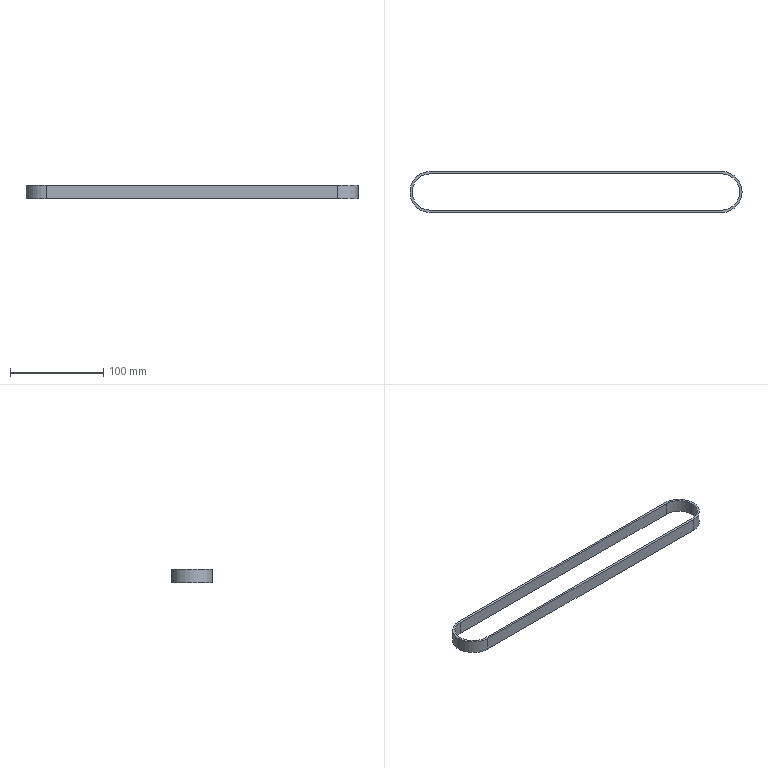Part | NX | features BREP 1 | 1 solid | 12 faces | box 356 x 44 x 14 mm | volume 26403 mm3 | cylinder 6 | plane 6 | commonest cylinder face diameters 39 x3 44 x3
STEP:
#1=CARTESIAN_POINT('',(256.,-22.,0.));
#2=VERTEX_POINT('',#1);
#3=CARTESIAN_POINT('',(278.,0.,0.));
#4=VERTEX_POINT('',#3);
#5=CARTESIAN_POINT('',(256.,0.,0.));
#6=DIRECTION('',(0.,0.,1.));
#7=DIRECTION('',(1.,0.,0.));
#8=AXIS2_PLACEMENT_3D('',#5,#6,#7);
#9=CIRCLE('',#8,22.);
#10=EDGE_CURVE('',#2,#4,#9,.T.);
#11=ORIENTED_EDGE('',*,*,#10,.T.);
#12=CARTESIAN_POINT('',(278.,0.,14.));
#13=VERTEX_POINT('',#12);
#14=CARTESIAN_POINT('',(278.,0.,0.));
#15=DIRECTION('',(0.,0.,1.));
#16=VECTOR('',#15,1000.);
#17=LINE('',#14,#16);
#18=EDGE_CURVE('',#4,#13,#17,.T.);
#19=ORIENTED_EDGE('',*,*,#18,.T.);
#20=CARTESIAN_POINT('',(256.,-22.,14.));
#21=VERTEX_POINT('',#20);
#22=CARTESIAN_POINT('',(256.,0.,14.));
#23=DIRECTION('',(0.,0.,1.));
#24=DIRECTION('',(1.,0.,0.));
#25=AXIS2_PLACEMENT_3D('',#22,#23,#24);
#26=CIRCLE('',#25,22.);
#27=EDGE_CURVE('',#21,#13,#26,.T.);
#28=ORIENTED_EDGE('',*,*,#27,.F.);
#29=CARTESIAN_POINT('',(256.,-22.,0.));
#30=DIRECTION('',(0.,0.,1.));
#31=VECTOR('',#30,1000.);
#32=LINE('',#29,#31);
#33=EDGE_CURVE('',#2,#21,#32,.T.);
#34=ORIENTED_EDGE('',*,*,#33,.F.);
#35=EDGE_LOOP('',(#11,#19,#28,#34));
#36=FACE_BOUND('',#35,.T.);
#37=CARTESIAN_POINT('',(256.,0.,0.));
#38=DIRECTION('',(0.,0.,1.));
#39=DIRECTION('',(1.,0.,0.));
#40=AXIS2_PLACEMENT_3D('',#37,#38,#39);
#41=CYLINDRICAL_SURFACE('',#40,22.);
#42=ADVANCED_FACE('',(#36),#41,.T.);
#43=CARTESIAN_POINT('',(256.,19.5,0.));
#44=VERTEX_POINT('',#43);
#45=CARTESIAN_POINT('',(275.5,0.,0.));
#46=VERTEX_POINT('',#45);
#47=CARTESIAN_POINT('',(256.,0.,0.));
#48=DIRECTION('',(0.,0.,-1.));
#49=DIRECTION('',(1.,0.,0.));
#50=AXIS2_PLACEMENT_3D('',#47,#48,#49);
#51=CIRCLE('',#50,19.5);
#52=EDGE_CURVE('',#44,#46,#51,.T.);
#53=ORIENTED_EDGE('',*,*,#52,.T.);
#54=CARTESIAN_POINT('',(275.5,0.,14.));
#55=VERTEX_POINT('',#54);
#56=CARTESIAN_POINT('',(275.5,0.,0.));
#57=DIRECTION('',(0.,0.,1.));
#58=VECTOR('',#57,1000.);
#59=LINE('',#56,#58);
#60=EDGE_CURVE('',#46,#55,#59,.T.);
#61=ORIENTED_EDGE('',*,*,#60,.T.);
#62=CARTESIAN_POINT('',(256.,19.5,14.));
#63=VERTEX_POINT('',#62);
#64=CARTESIAN_POINT('',(256.,0.,14.));
#65=DIRECTION('',(0.,0.,-1.));
#66=DIRECTION('',(1.,0.,0.));
#67=AXIS2_PLACEMENT_3D('',#64,#65,#66);
#68=CIRCLE('',#67,19.5);
#69=EDGE_CURVE('',#63,#55,#68,.T.);
#70=ORIENTED_EDGE('',*,*,#69,.F.);
#71=CARTESIAN_POINT('',(256.,19.5,0.));
#72=DIRECTION('',(0.,0.,-1.));
#73=VECTOR('',#72,1000.);
#74=LINE('',#71,#73);
#75=EDGE_CURVE('',#63,#44,#74,.T.);
#76=ORIENTED_EDGE('',*,*,#75,.T.);
#77=EDGE_LOOP('',(#53,#61,#70,#76));
#78=FACE_BOUND('',#77,.T.);
#79=CARTESIAN_POINT('',(256.,0.,0.));
#80=DIRECTION('',(0.,0.,1.));
#81=DIRECTION('',(1.,0.,0.));
#82=AXIS2_PLACEMENT_3D('',#79,#80,#81);
#83=CYLINDRICAL_SURFACE('',#82,19.5);
#84=ADVANCED_FACE('',(#78),#83,.F.);
#85=CARTESIAN_POINT('',(-56.,-22.,0.));
#86=VERTEX_POINT('',#85);
#87=CARTESIAN_POINT('',(0.,-22.,0.));
#88=DIRECTION('',(-1.,0.,0.));
#89=VECTOR('',#88,1000.);
#90=LINE('',#87,#89);
#91=EDGE_CURVE('',#2,#86,#90,.T.);
#92=ORIENTED_EDGE('',*,*,#91,.T.);
#93=CARTESIAN_POINT('',(-56.,22.,0.));
#94=VERTEX_POINT('',#93);
#95=CARTESIAN_POINT('',(-56.,0.,0.));
#96=DIRECTION('',(0.,0.,1.));
#97=DIRECTION('',(1.,0.,0.));
#98=AXIS2_PLACEMENT_3D('',#95,#96,#97);
#99=CIRCLE('',#98,22.);
#100=EDGE_CURVE('',#94,#86,#99,.T.);
#101=ORIENTED_EDGE('',*,*,#100,.F.);
#102=CARTESIAN_POINT('',(256.,22.,0.));
#103=VERTEX_POINT('',#102);
#104=CARTESIAN_POINT('',(0.,22.,0.));
#105=DIRECTION('',(1.,0.,0.));
#106=VECTOR('',#105,1000.);
#107=LINE('',#104,#106);
#108=EDGE_CURVE('',#94,#103,#107,.T.);
#109=ORIENTED_EDGE('',*,*,#108,.T.);
#110=CARTESIAN_POINT('',(256.,0.,0.));
#111=DIRECTION('',(0.,0.,1.));
#112=DIRECTION('',(1.,0.,0.));
#113=AXIS2_PLACEMENT_3D('',#110,#111,#112);
#114=CIRCLE('',#113,22.);
#115=EDGE_CURVE('',#4,#103,#114,.T.);
#116=ORIENTED_EDGE('',*,*,#115,.F.);
#117=ORIENTED_EDGE('',*,*,#10,.F.);
#118=EDGE_LOOP('',(#92,#101,#109,#116,#117));
#119=FACE_BOUND('',#118,.T.);
#120=CARTESIAN_POINT('',(-56.,-19.5,0.));
#121=VERTEX_POINT('',#120);
#122=CARTESIAN_POINT('',(-56.,19.5,0.));
#123=VERTEX_POINT('',#122);
#124=CARTESIAN_POINT('',(-56.,0.,0.));
#125=DIRECTION('',(0.,0.,-1.));
#126=DIRECTION('',(1.,0.,0.));
#127=AXIS2_PLACEMENT_3D('',#124,#125,#126);
#128=CIRCLE('',#127,19.5);
#129=EDGE_CURVE('',#121,#123,#128,.T.);
#130=ORIENTED_EDGE('',*,*,#129,.F.);
#131=CARTESIAN_POINT('',(256.,-19.5,0.));
#132=VERTEX_POINT('',#131);
#133=CARTESIAN_POINT('',(0.,-19.5,0.));
#134=DIRECTION('',(-1.,0.,0.));
#135=VECTOR('',#134,1000.);
#136=LINE('',#133,#135);
#137=EDGE_CURVE('',#132,#121,#136,.T.);
#138=ORIENTED_EDGE('',*,*,#137,.F.);
#139=CARTESIAN_POINT('',(256.,0.,0.));
#140=DIRECTION('',(0.,0.,-1.));
#141=DIRECTION('',(1.,0.,0.));
#142=AXIS2_PLACEMENT_3D('',#139,#140,#141);
#143=CIRCLE('',#142,19.5);
#144=EDGE_CURVE('',#46,#132,#143,.T.);
#145=ORIENTED_EDGE('',*,*,#144,.F.);
#146=ORIENTED_EDGE('',*,*,#52,.F.);
#147=CARTESIAN_POINT('',(0.,19.5,0.));
#148=DIRECTION('',(1.,0.,0.));
#149=VECTOR('',#148,1000.);
#150=LINE('',#147,#149);
#151=EDGE_CURVE('',#123,#44,#150,.T.);
#152=ORIENTED_EDGE('',*,*,#151,.F.);
#153=EDGE_LOOP('',(#130,#138,#145,#146,#152));
#154=FACE_BOUND('',#153,.T.);
#155=CARTESIAN_POINT('',(0.,0.,0.));
#156=DIRECTION('',(0.,0.,1.));
#157=DIRECTION('',(1.,0.,0.));
#158=AXIS2_PLACEMENT_3D('',#155,#156,#157);
#159=PLANE('',#158);
#160=ADVANCED_FACE('',(#119,#154),#159,.F.);
#161=CARTESIAN_POINT('',(-56.,-22.,14.));
#162=VERTEX_POINT('',#161);
#163=CARTESIAN_POINT('',(0.,-22.,14.));
#164=DIRECTION('',(-1.,0.,0.));
#165=VECTOR('',#164,1000.);
#166=LINE('',#163,#165);
#167=EDGE_CURVE('',#21,#162,#166,.T.);
#168=ORIENTED_EDGE('',*,*,#167,.F.);
#169=ORIENTED_EDGE('',*,*,#27,.T.);
#170=CARTESIAN_POINT('',(256.,22.,14.));
#171=VERTEX_POINT('',#170);
#172=CARTESIAN_POINT('',(256.,0.,14.));
#173=DIRECTION('',(0.,0.,1.));
#174=DIRECTION('',(1.,0.,0.));
#175=AXIS2_PLACEMENT_3D('',#172,#173,#174);
#176=CIRCLE('',#175,22.);
#177=EDGE_CURVE('',#13,#171,#176,.T.);
#178=ORIENTED_EDGE('',*,*,#177,.T.);
#179=CARTESIAN_POINT('',(-56.,22.,14.));
#180=VERTEX_POINT('',#179);
#181=CARTESIAN_POINT('',(0.,22.,14.));
#182=DIRECTION('',(1.,0.,0.));
#183=VECTOR('',#182,1000.);
#184=LINE('',#181,#183);
#185=EDGE_CURVE('',#180,#171,#184,.T.);
#186=ORIENTED_EDGE('',*,*,#185,.F.);
#187=CARTESIAN_POINT('',(-56.,0.,14.));
#188=DIRECTION('',(0.,0.,1.));
#189=DIRECTION('',(1.,0.,0.));
#190=AXIS2_PLACEMENT_3D('',#187,#188,#189);
#191=CIRCLE('',#190,22.);
#192=EDGE_CURVE('',#180,#162,#191,.T.);
#193=ORIENTED_EDGE('',*,*,#192,.T.);
#194=EDGE_LOOP('',(#168,#169,#178,#186,#193));
#195=FACE_BOUND('',#194,.T.);
#196=ORIENTED_EDGE('',*,*,#69,.T.);
#197=CARTESIAN_POINT('',(256.,-19.5,14.));
#198=VERTEX_POINT('',#197);
#199=CARTESIAN_POINT('',(256.,0.,14.));
#200=DIRECTION('',(0.,0.,-1.));
#201=DIRECTION('',(1.,0.,0.));
#202=AXIS2_PLACEMENT_3D('',#199,#200,#201);
#203=CIRCLE('',#202,19.5);
#204=EDGE_CURVE('',#55,#198,#203,.T.);
#205=ORIENTED_EDGE('',*,*,#204,.T.);
#206=CARTESIAN_POINT('',(-56.,-19.5,14.));
#207=VERTEX_POINT('',#206);
#208=CARTESIAN_POINT('',(0.,-19.5,14.));
#209=DIRECTION('',(-1.,0.,0.));
#210=VECTOR('',#209,1000.);
#211=LINE('',#208,#210);
#212=EDGE_CURVE('',#198,#207,#211,.T.);
#213=ORIENTED_EDGE('',*,*,#212,.T.);
#214=CARTESIAN_POINT('',(-56.,19.5,14.));
#215=VERTEX_POINT('',#214);
#216=CARTESIAN_POINT('',(-56.,0.,14.));
#217=DIRECTION('',(0.,0.,-1.));
#218=DIRECTION('',(1.,0.,0.));
#219=AXIS2_PLACEMENT_3D('',#216,#217,#218);
#220=CIRCLE('',#219,19.5);
#221=EDGE_CURVE('',#207,#215,#220,.T.);
#222=ORIENTED_EDGE('',*,*,#221,.T.);
#223=CARTESIAN_POINT('',(0.,19.5,14.));
#224=DIRECTION('',(1.,0.,0.));
#225=VECTOR('',#224,1000.);
#226=LINE('',#223,#225);
#227=EDGE_CURVE('',#215,#63,#226,.T.);
#228=ORIENTED_EDGE('',*,*,#227,.T.);
#229=EDGE_LOOP('',(#196,#205,#213,#222,#228));
#230=FACE_BOUND('',#229,.T.);
#231=CARTESIAN_POINT('',(0.,0.,14.));
#232=DIRECTION('',(0.,0.,1.));
#233=DIRECTION('',(1.,0.,0.));
#234=AXIS2_PLACEMENT_3D('',#231,#232,#233);
#235=PLANE('',#234);
#236=ADVANCED_FACE('',(#195,#230),#235,.T.);
#237=CARTESIAN_POINT('',(-56.,19.5,0.));
#238=DIRECTION('',(0.,0.,1.));
#239=VECTOR('',#238,1000.);
#240=LINE('',#237,#239);
#241=EDGE_CURVE('',#123,#215,#240,.T.);
#242=ORIENTED_EDGE('',*,*,#241,.F.);
#243=ORIENTED_EDGE('',*,*,#151,.T.);
#244=ORIENTED_EDGE('',*,*,#75,.F.);
#245=ORIENTED_EDGE('',*,*,#227,.F.);
#246=EDGE_LOOP('',(#242,#243,#244,#245));
#247=FACE_BOUND('',#246,.T.);
#248=CARTESIAN_POINT('',(0.,19.5,0.));
#249=DIRECTION('',(0.,1.,0.));
#250=DIRECTION('',(1.,0.,0.));
#251=AXIS2_PLACEMENT_3D('',#248,#249,#250);
#252=PLANE('',#251);
#253=ADVANCED_FACE('',(#247),#252,.F.);
#254=CARTESIAN_POINT('',(-56.,-19.5,0.));
#255=DIRECTION('',(0.,0.,1.));
#256=VECTOR('',#255,1000.);
#257=LINE('',#254,#256);
#258=EDGE_CURVE('',#121,#207,#257,.T.);
#259=ORIENTED_EDGE('',*,*,#258,.F.);
#260=ORIENTED_EDGE('',*,*,#129,.T.);
#261=ORIENTED_EDGE('',*,*,#241,.T.);
#262=ORIENTED_EDGE('',*,*,#221,.F.);
#263=EDGE_LOOP('',(#259,#260,#261,#262));
#264=FACE_BOUND('',#263,.T.);
#265=CARTESIAN_POINT('',(-56.,0.,0.));
#266=DIRECTION('',(0.,0.,1.));
#267=DIRECTION('',(1.,0.,0.));
#268=AXIS2_PLACEMENT_3D('',#265,#266,#267);
#269=CYLINDRICAL_SURFACE('',#268,19.5);
#270=ADVANCED_FACE('',(#264),#269,.F.);
#271=CARTESIAN_POINT('',(256.,-19.5,0.));
#272=DIRECTION('',(0.,0.,1.));
#273=VECTOR('',#272,1000.);
#274=LINE('',#271,#273);
#275=EDGE_CURVE('',#132,#198,#274,.T.);
#276=ORIENTED_EDGE('',*,*,#275,.F.);
#277=ORIENTED_EDGE('',*,*,#137,.T.);
#278=ORIENTED_EDGE('',*,*,#258,.T.);
#279=ORIENTED_EDGE('',*,*,#212,.F.);
#280=EDGE_LOOP('',(#276,#277,#278,#279));
#281=FACE_BOUND('',#280,.T.);
#282=CARTESIAN_POINT('',(0.,-19.5,0.));
#283=DIRECTION('',(0.,-1.,0.));
#284=DIRECTION('',(0.,0.,-1.));
#285=AXIS2_PLACEMENT_3D('',#282,#283,#284);
#286=PLANE('',#285);
#287=ADVANCED_FACE('',(#281),#286,.F.);
#288=ORIENTED_EDGE('',*,*,#60,.F.);
#289=ORIENTED_EDGE('',*,*,#144,.T.);
#290=ORIENTED_EDGE('',*,*,#275,.T.);
#291=ORIENTED_EDGE('',*,*,#204,.F.);
#292=EDGE_LOOP('',(#288,#289,#290,#291));
#293=FACE_BOUND('',#292,.T.);
#294=CARTESIAN_POINT('',(256.,0.,0.));
#295=DIRECTION('',(0.,0.,1.));
#296=DIRECTION('',(1.,0.,0.));
#297=AXIS2_PLACEMENT_3D('',#294,#295,#296);
#298=CYLINDRICAL_SURFACE('',#297,19.5);
#299=ADVANCED_FACE('',(#293),#298,.F.);
#300=ORIENTED_EDGE('',*,*,#167,.T.);
#301=CARTESIAN_POINT('',(-56.,-22.,0.));
#302=DIRECTION('',(0.,0.,1.));
#303=VECTOR('',#302,1000.);
#304=LINE('',#301,#303);
#305=EDGE_CURVE('',#86,#162,#304,.T.);
#306=ORIENTED_EDGE('',*,*,#305,.F.);
#307=ORIENTED_EDGE('',*,*,#91,.F.);
#308=ORIENTED_EDGE('',*,*,#33,.T.);
#309=EDGE_LOOP('',(#300,#306,#307,#308));
#310=FACE_BOUND('',#309,.T.);
#311=CARTESIAN_POINT('',(0.,-22.,0.));
#312=DIRECTION('',(0.,1.,0.));
#313=DIRECTION('',(1.,0.,0.));
#314=AXIS2_PLACEMENT_3D('',#311,#312,#313);
#315=PLANE('',#314);
#316=ADVANCED_FACE('',(#310),#315,.F.);
#317=ORIENTED_EDGE('',*,*,#192,.F.);
#318=CARTESIAN_POINT('',(-56.,22.,0.));
#319=DIRECTION('',(0.,0.,1.));
#320=VECTOR('',#319,1000.);
#321=LINE('',#318,#320);
#322=EDGE_CURVE('',#94,#180,#321,.T.);
#323=ORIENTED_EDGE('',*,*,#322,.F.);
#324=ORIENTED_EDGE('',*,*,#100,.T.);
#325=ORIENTED_EDGE('',*,*,#305,.T.);
#326=EDGE_LOOP('',(#317,#323,#324,#325));
#327=FACE_BOUND('',#326,.T.);
#328=CARTESIAN_POINT('',(-56.,0.,0.));
#329=DIRECTION('',(0.,0.,1.));
#330=DIRECTION('',(1.,0.,0.));
#331=AXIS2_PLACEMENT_3D('',#328,#329,#330);
#332=CYLINDRICAL_SURFACE('',#331,22.);
#333=ADVANCED_FACE('',(#327),#332,.T.);
#334=ORIENTED_EDGE('',*,*,#185,.T.);
#335=CARTESIAN_POINT('',(256.,22.,0.));
#336=DIRECTION('',(0.,0.,1.));
#337=VECTOR('',#336,1000.);
#338=LINE('',#335,#337);
#339=EDGE_CURVE('',#103,#171,#338,.T.);
#340=ORIENTED_EDGE('',*,*,#339,.F.);
#341=ORIENTED_EDGE('',*,*,#108,.F.);
#342=ORIENTED_EDGE('',*,*,#322,.T.);
#343=EDGE_LOOP('',(#334,#340,#341,#342));
#344=FACE_BOUND('',#343,.T.);
#345=CARTESIAN_POINT('',(0.,22.,0.));
#346=DIRECTION('',(0.,-1.,0.));
#347=DIRECTION('',(0.,0.,-1.));
#348=AXIS2_PLACEMENT_3D('',#345,#346,#347);
#349=PLANE('',#348);
#350=ADVANCED_FACE('',(#344),#349,.F.);
#351=ORIENTED_EDGE('',*,*,#18,.F.);
#352=ORIENTED_EDGE('',*,*,#115,.T.);
#353=ORIENTED_EDGE('',*,*,#339,.T.);
#354=ORIENTED_EDGE('',*,*,#177,.F.);
#355=EDGE_LOOP('',(#351,#352,#353,#354));
#356=FACE_BOUND('',#355,.T.);
#357=CARTESIAN_POINT('',(256.,0.,0.));
#358=DIRECTION('',(0.,0.,1.));
#359=DIRECTION('',(1.,0.,0.));
#360=AXIS2_PLACEMENT_3D('',#357,#358,#359);
#361=CYLINDRICAL_SURFACE('',#360,22.);
#362=ADVANCED_FACE('',(#356),#361,.T.);
#363=CLOSED_SHELL('',(#42,#84,#160,#236,#253,#270,#287,#299,#316,#333,#350,#362));
#364=MANIFOLD_SOLID_BREP('',#363);
#365=(LENGTH_UNIT()NAMED_UNIT(*)SI_UNIT(.MILLI.,.METRE.));
#366=UNCERTAINTY_MEASURE_WITH_UNIT(LENGTH_MEASURE(0.00001),#365,'','');
#367=(NAMED_UNIT(*)PLANE_ANGLE_UNIT()SI_UNIT($,.RADIAN.));
#368=(NAMED_UNIT(*)SI_UNIT($,.STERADIAN.)SOLID_ANGLE_UNIT());
#369=(GEOMETRIC_REPRESENTATION_CONTEXT(3)GLOBAL_UNCERTAINTY_ASSIGNED_CONTEXT((#366))GLOBAL_UNIT_ASSIGNED_CONTEXT((#365,#367,#368))REPRESENTATION_CONTEXT('',''));
#370=ADVANCED_BREP_SHAPE_REPRESENTATION('',(#364),#369);